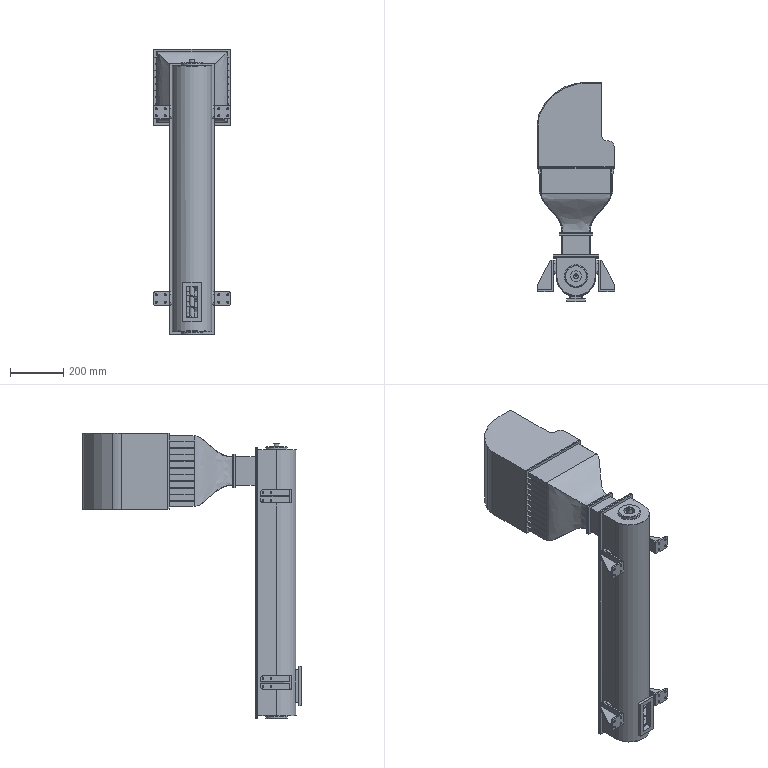Part | STEP file | Screew Feeder | 10 solids | 490 faces | box 290 x 822.474 x 1075 mm | volume 4769697 mm3 | plane 352 | cylinder 121 | spline 12 | cone 3 | torus 2 | commonest cylinder face diameters 20 x50 6 x32 8 x16 10 x8 40 x4 42 x2